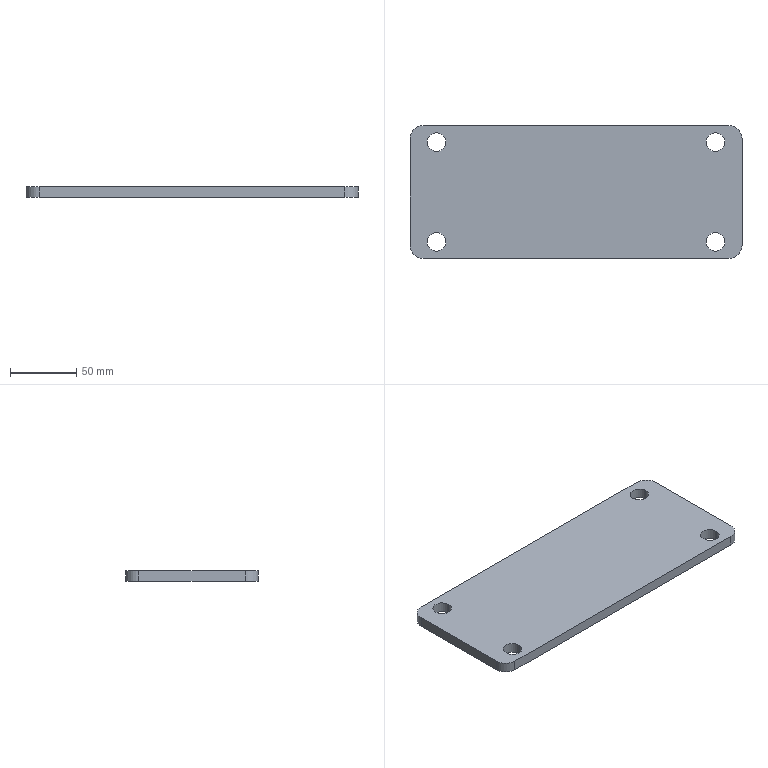Part | SolidWorks | features Chamfer 1, Extrusion 1, Fillet 1, HoleWzd 1 | 1 solid | 18 faces | box 250 x 100 x 8 mm | volume 194387 mm3 | cylinder 12 | plane 6 | commonest cylinder face diameters 14 x8 20 x4
STEP:
#1=CARTESIAN_POINT('',(-112.,37.5,-4.));
#2=VERTEX_POINT('',#1);
#3=CARTESIAN_POINT('',(-98.,37.5,-4.));
#4=VERTEX_POINT('',#3);
#5=CARTESIAN_POINT('',(-105.,37.5,-4.));
#6=DIRECTION('',(0.,0.,1.));
#7=DIRECTION('',(1.,0.,0.));
#8=AXIS2_PLACEMENT_3D('',#5,#6,#7);
#9=CIRCLE('',#8,7.);
#10=EDGE_CURVE('',#2,#4,#9,.T.);
#11=ORIENTED_EDGE('',*,*,#10,.F.);
#12=CARTESIAN_POINT('',(-112.,37.5,4.));
#13=VERTEX_POINT('',#12);
#14=CARTESIAN_POINT('',(-112.,37.5,4.));
#15=DIRECTION('',(0.,0.,1.));
#16=VECTOR('',#15,1000.);
#17=LINE('',#14,#16);
#18=EDGE_CURVE('',#2,#13,#17,.T.);
#19=ORIENTED_EDGE('',*,*,#18,.T.);
#20=CARTESIAN_POINT('',(-98.,37.5,4.));
#21=VERTEX_POINT('',#20);
#22=CARTESIAN_POINT('',(-105.,37.5,4.));
#23=DIRECTION('',(0.,0.,1.));
#24=DIRECTION('',(1.,0.,0.));
#25=AXIS2_PLACEMENT_3D('',#22,#23,#24);
#26=CIRCLE('',#25,7.);
#27=EDGE_CURVE('',#13,#21,#26,.T.);
#28=ORIENTED_EDGE('',*,*,#27,.T.);
#29=CARTESIAN_POINT('',(-98.,37.5,4.));
#30=DIRECTION('',(0.,0.,1.));
#31=VECTOR('',#30,1000.);
#32=LINE('',#29,#31);
#33=EDGE_CURVE('',#4,#21,#32,.T.);
#34=ORIENTED_EDGE('',*,*,#33,.F.);
#35=EDGE_LOOP('',(#11,#19,#28,#34));
#36=FACE_OUTER_BOUND('',#35,.T.);
#37=CARTESIAN_POINT('',(-105.,37.5,4.));
#38=DIRECTION('',(0.,0.,1.));
#39=DIRECTION('',(1.,0.,0.));
#40=AXIS2_PLACEMENT_3D('',#37,#38,#39);
#41=CYLINDRICAL_SURFACE('',#40,7.);
#42=ADVANCED_FACE('',(#36),#41,.F.);
#43=CARTESIAN_POINT('',(98.,37.5,-4.));
#44=VERTEX_POINT('',#43);
#45=CARTESIAN_POINT('',(112.,37.5,-4.));
#46=VERTEX_POINT('',#45);
#47=CARTESIAN_POINT('',(105.,37.5,-4.));
#48=DIRECTION('',(0.,0.,1.));
#49=DIRECTION('',(1.,0.,0.));
#50=AXIS2_PLACEMENT_3D('',#47,#48,#49);
#51=CIRCLE('',#50,7.);
#52=EDGE_CURVE('',#44,#46,#51,.T.);
#53=ORIENTED_EDGE('',*,*,#52,.F.);
#54=CARTESIAN_POINT('',(98.,37.5,4.));
#55=VERTEX_POINT('',#54);
#56=CARTESIAN_POINT('',(98.,37.5,4.));
#57=DIRECTION('',(0.,0.,1.));
#58=VECTOR('',#57,1000.);
#59=LINE('',#56,#58);
#60=EDGE_CURVE('',#44,#55,#59,.T.);
#61=ORIENTED_EDGE('',*,*,#60,.T.);
#62=CARTESIAN_POINT('',(112.,37.5,4.));
#63=VERTEX_POINT('',#62);
#64=CARTESIAN_POINT('',(105.,37.5,4.));
#65=DIRECTION('',(0.,0.,1.));
#66=DIRECTION('',(1.,0.,0.));
#67=AXIS2_PLACEMENT_3D('',#64,#65,#66);
#68=CIRCLE('',#67,7.);
#69=EDGE_CURVE('',#55,#63,#68,.T.);
#70=ORIENTED_EDGE('',*,*,#69,.T.);
#71=CARTESIAN_POINT('',(112.,37.5,4.));
#72=DIRECTION('',(0.,0.,1.));
#73=VECTOR('',#72,1000.);
#74=LINE('',#71,#73);
#75=EDGE_CURVE('',#46,#63,#74,.T.);
#76=ORIENTED_EDGE('',*,*,#75,.F.);
#77=EDGE_LOOP('',(#53,#61,#70,#76));
#78=FACE_OUTER_BOUND('',#77,.T.);
#79=CARTESIAN_POINT('',(105.,37.5,4.));
#80=DIRECTION('',(0.,0.,1.));
#81=DIRECTION('',(1.,0.,0.));
#82=AXIS2_PLACEMENT_3D('',#79,#80,#81);
#83=CYLINDRICAL_SURFACE('',#82,7.);
#84=ADVANCED_FACE('',(#78),#83,.F.);
#85=CARTESIAN_POINT('',(98.,-37.5,-4.));
#86=VERTEX_POINT('',#85);
#87=CARTESIAN_POINT('',(112.,-37.5,-4.));
#88=VERTEX_POINT('',#87);
#89=CARTESIAN_POINT('',(105.,-37.5,-4.));
#90=DIRECTION('',(0.,0.,1.));
#91=DIRECTION('',(1.,0.,0.));
#92=AXIS2_PLACEMENT_3D('',#89,#90,#91);
#93=CIRCLE('',#92,7.);
#94=EDGE_CURVE('',#86,#88,#93,.T.);
#95=ORIENTED_EDGE('',*,*,#94,.F.);
#96=CARTESIAN_POINT('',(98.,-37.5,4.));
#97=VERTEX_POINT('',#96);
#98=CARTESIAN_POINT('',(98.,-37.5,4.));
#99=DIRECTION('',(0.,0.,1.));
#100=VECTOR('',#99,1000.);
#101=LINE('',#98,#100);
#102=EDGE_CURVE('',#86,#97,#101,.T.);
#103=ORIENTED_EDGE('',*,*,#102,.T.);
#104=CARTESIAN_POINT('',(112.,-37.5,4.));
#105=VERTEX_POINT('',#104);
#106=CARTESIAN_POINT('',(105.,-37.5,4.));
#107=DIRECTION('',(0.,0.,1.));
#108=DIRECTION('',(1.,0.,0.));
#109=AXIS2_PLACEMENT_3D('',#106,#107,#108);
#110=CIRCLE('',#109,7.);
#111=EDGE_CURVE('',#97,#105,#110,.T.);
#112=ORIENTED_EDGE('',*,*,#111,.T.);
#113=CARTESIAN_POINT('',(112.,-37.5,4.));
#114=DIRECTION('',(0.,0.,1.));
#115=VECTOR('',#114,1000.);
#116=LINE('',#113,#115);
#117=EDGE_CURVE('',#88,#105,#116,.T.);
#118=ORIENTED_EDGE('',*,*,#117,.F.);
#119=EDGE_LOOP('',(#95,#103,#112,#118));
#120=FACE_OUTER_BOUND('',#119,.T.);
#121=CARTESIAN_POINT('',(105.,-37.5,4.));
#122=DIRECTION('',(0.,0.,1.));
#123=DIRECTION('',(1.,0.,0.));
#124=AXIS2_PLACEMENT_3D('',#121,#122,#123);
#125=CYLINDRICAL_SURFACE('',#124,7.);
#126=ADVANCED_FACE('',(#120),#125,.F.);
#127=CARTESIAN_POINT('',(-112.,-37.5,-4.));
#128=VERTEX_POINT('',#127);
#129=CARTESIAN_POINT('',(-98.,-37.5,-4.));
#130=VERTEX_POINT('',#129);
#131=CARTESIAN_POINT('',(-105.,-37.5,-4.));
#132=DIRECTION('',(0.,0.,1.));
#133=DIRECTION('',(1.,0.,0.));
#134=AXIS2_PLACEMENT_3D('',#131,#132,#133);
#135=CIRCLE('',#134,7.);
#136=EDGE_CURVE('',#128,#130,#135,.T.);
#137=ORIENTED_EDGE('',*,*,#136,.F.);
#138=CARTESIAN_POINT('',(-112.,-37.5,4.));
#139=VERTEX_POINT('',#138);
#140=CARTESIAN_POINT('',(-112.,-37.5,4.));
#141=DIRECTION('',(0.,0.,1.));
#142=VECTOR('',#141,1000.);
#143=LINE('',#140,#142);
#144=EDGE_CURVE('',#128,#139,#143,.T.);
#145=ORIENTED_EDGE('',*,*,#144,.T.);
#146=CARTESIAN_POINT('',(-98.,-37.5,4.));
#147=VERTEX_POINT('',#146);
#148=CARTESIAN_POINT('',(-105.,-37.5,4.));
#149=DIRECTION('',(0.,0.,1.));
#150=DIRECTION('',(1.,0.,0.));
#151=AXIS2_PLACEMENT_3D('',#148,#149,#150);
#152=CIRCLE('',#151,7.);
#153=EDGE_CURVE('',#139,#147,#152,.T.);
#154=ORIENTED_EDGE('',*,*,#153,.T.);
#155=CARTESIAN_POINT('',(-98.,-37.5,4.));
#156=DIRECTION('',(0.,0.,1.));
#157=VECTOR('',#156,1000.);
#158=LINE('',#155,#157);
#159=EDGE_CURVE('',#130,#147,#158,.T.);
#160=ORIENTED_EDGE('',*,*,#159,.F.);
#161=EDGE_LOOP('',(#137,#145,#154,#160));
#162=FACE_OUTER_BOUND('',#161,.T.);
#163=CARTESIAN_POINT('',(-105.,-37.5,4.));
#164=DIRECTION('',(0.,0.,1.));
#165=DIRECTION('',(1.,0.,0.));
#166=AXIS2_PLACEMENT_3D('',#163,#164,#165);
#167=CYLINDRICAL_SURFACE('',#166,7.);
#168=ADVANCED_FACE('',(#162),#167,.F.);
#169=CARTESIAN_POINT('',(-125.,40.,-4.));
#170=VERTEX_POINT('',#169);
#171=CARTESIAN_POINT('',(-125.,-40.,-4.));
#172=VERTEX_POINT('',#171);
#173=CARTESIAN_POINT('',(-125.,-50.,-4.));
#174=DIRECTION('',(0.,-1.,0.));
#175=VECTOR('',#174,1000.);
#176=LINE('',#173,#175);
#177=EDGE_CURVE('',#170,#172,#176,.T.);
#178=ORIENTED_EDGE('',*,*,#177,.T.);
#179=CARTESIAN_POINT('',(-125.,-40.,4.));
#180=VERTEX_POINT('',#179);
#181=CARTESIAN_POINT('',(-125.,-40.,4.));
#182=DIRECTION('',(0.,0.,1.));
#183=VECTOR('',#182,1000.);
#184=LINE('',#181,#183);
#185=EDGE_CURVE('',#172,#180,#184,.T.);
#186=ORIENTED_EDGE('',*,*,#185,.T.);
#187=CARTESIAN_POINT('',(-125.,40.,4.));
#188=VERTEX_POINT('',#187);
#189=CARTESIAN_POINT('',(-125.,-50.,4.));
#190=DIRECTION('',(0.,-1.,0.));
#191=VECTOR('',#190,1000.);
#192=LINE('',#189,#191);
#193=EDGE_CURVE('',#188,#180,#192,.T.);
#194=ORIENTED_EDGE('',*,*,#193,.F.);
#195=CARTESIAN_POINT('',(-125.,40.,4.));
#196=DIRECTION('',(0.,0.,-1.));
#197=VECTOR('',#196,1000.);
#198=LINE('',#195,#197);
#199=EDGE_CURVE('',#188,#170,#198,.T.);
#200=ORIENTED_EDGE('',*,*,#199,.T.);
#201=EDGE_LOOP('',(#178,#186,#194,#200));
#202=FACE_OUTER_BOUND('',#201,.T.);
#203=CARTESIAN_POINT('',(-125.,-50.,4.));
#204=DIRECTION('',(1.,0.,0.));
#205=DIRECTION('',(0.,0.,-1.));
#206=AXIS2_PLACEMENT_3D('',#203,#204,#205);
#207=PLANE('',#206);
#208=ADVANCED_FACE('',(#202),#207,.F.);
#209=CARTESIAN_POINT('',(-115.,-50.,-4.));
#210=VERTEX_POINT('',#209);
#211=CARTESIAN_POINT('',(115.,-50.,-4.));
#212=VERTEX_POINT('',#211);
#213=CARTESIAN_POINT('',(125.,-50.,-4.));
#214=DIRECTION('',(1.,0.,0.));
#215=VECTOR('',#214,1000.);
#216=LINE('',#213,#215);
#217=EDGE_CURVE('',#210,#212,#216,.T.);
#218=ORIENTED_EDGE('',*,*,#217,.T.);
#219=CARTESIAN_POINT('',(115.,-50.,4.));
#220=VERTEX_POINT('',#219);
#221=CARTESIAN_POINT('',(115.,-50.,4.));
#222=DIRECTION('',(0.,0.,1.));
#223=VECTOR('',#222,1000.);
#224=LINE('',#221,#223);
#225=EDGE_CURVE('',#212,#220,#224,.T.);
#226=ORIENTED_EDGE('',*,*,#225,.T.);
#227=CARTESIAN_POINT('',(-115.,-50.,4.));
#228=VERTEX_POINT('',#227);
#229=CARTESIAN_POINT('',(125.,-50.,4.));
#230=DIRECTION('',(1.,0.,0.));
#231=VECTOR('',#230,1000.);
#232=LINE('',#229,#231);
#233=EDGE_CURVE('',#228,#220,#232,.T.);
#234=ORIENTED_EDGE('',*,*,#233,.F.);
#235=CARTESIAN_POINT('',(-115.,-50.,4.));
#236=DIRECTION('',(0.,0.,-1.));
#237=VECTOR('',#236,1000.);
#238=LINE('',#235,#237);
#239=EDGE_CURVE('',#228,#210,#238,.T.);
#240=ORIENTED_EDGE('',*,*,#239,.T.);
#241=EDGE_LOOP('',(#218,#226,#234,#240));
#242=FACE_OUTER_BOUND('',#241,.T.);
#243=CARTESIAN_POINT('',(125.,-50.,4.));
#244=DIRECTION('',(0.,1.,0.));
#245=DIRECTION('',(-1.,0.,0.));
#246=AXIS2_PLACEMENT_3D('',#243,#244,#245);
#247=PLANE('',#246);
#248=ADVANCED_FACE('',(#242),#247,.F.);
#249=CARTESIAN_POINT('',(125.,-40.,-4.));
#250=VERTEX_POINT('',#249);
#251=CARTESIAN_POINT('',(125.,40.,-4.));
#252=VERTEX_POINT('',#251);
#253=CARTESIAN_POINT('',(125.,-50.,-4.));
#254=DIRECTION('',(0.,1.,0.));
#255=VECTOR('',#254,1000.);
#256=LINE('',#253,#255);
#257=EDGE_CURVE('',#250,#252,#256,.T.);
#258=ORIENTED_EDGE('',*,*,#257,.T.);
#259=CARTESIAN_POINT('',(125.,40.,4.));
#260=VERTEX_POINT('',#259);
#261=CARTESIAN_POINT('',(125.,40.,4.));
#262=DIRECTION('',(0.,0.,1.));
#263=VECTOR('',#262,1000.);
#264=LINE('',#261,#263);
#265=EDGE_CURVE('',#252,#260,#264,.T.);
#266=ORIENTED_EDGE('',*,*,#265,.T.);
#267=CARTESIAN_POINT('',(125.,-40.,4.));
#268=VERTEX_POINT('',#267);
#269=CARTESIAN_POINT('',(125.,-50.,4.));
#270=DIRECTION('',(0.,1.,0.));
#271=VECTOR('',#270,1000.);
#272=LINE('',#269,#271);
#273=EDGE_CURVE('',#268,#260,#272,.T.);
#274=ORIENTED_EDGE('',*,*,#273,.F.);
#275=CARTESIAN_POINT('',(125.,-40.,4.));
#276=DIRECTION('',(0.,0.,-1.));
#277=VECTOR('',#276,1000.);
#278=LINE('',#275,#277);
#279=EDGE_CURVE('',#268,#250,#278,.T.);
#280=ORIENTED_EDGE('',*,*,#279,.T.);
#281=EDGE_LOOP('',(#258,#266,#274,#280));
#282=FACE_OUTER_BOUND('',#281,.T.);
#283=CARTESIAN_POINT('',(125.,-50.,4.));
#284=DIRECTION('',(-1.,0.,0.));
#285=DIRECTION('',(0.,0.,1.));
#286=AXIS2_PLACEMENT_3D('',#283,#284,#285);
#287=PLANE('',#286);
#288=ADVANCED_FACE('',(#282),#287,.F.);
#289=CARTESIAN_POINT('',(115.,50.,4.));
#290=VERTEX_POINT('',#289);
#291=CARTESIAN_POINT('',(-115.,50.,4.));
#292=VERTEX_POINT('',#291);
#293=CARTESIAN_POINT('',(125.,50.,4.));
#294=DIRECTION('',(-1.,0.,0.));
#295=VECTOR('',#294,1000.);
#296=LINE('',#293,#295);
#297=EDGE_CURVE('',#290,#292,#296,.T.);
#298=ORIENTED_EDGE('',*,*,#297,.F.);
#299=CARTESIAN_POINT('',(115.,50.,-4.));
#300=VERTEX_POINT('',#299);
#301=CARTESIAN_POINT('',(115.,50.,4.));
#302=DIRECTION('',(0.,0.,-1.));
#303=VECTOR('',#302,1000.);
#304=LINE('',#301,#303);
#305=EDGE_CURVE('',#290,#300,#304,.T.);
#306=ORIENTED_EDGE('',*,*,#305,.T.);
#307=CARTESIAN_POINT('',(-115.,50.,-4.));
#308=VERTEX_POINT('',#307);
#309=CARTESIAN_POINT('',(125.,50.,-4.));
#310=DIRECTION('',(-1.,0.,0.));
#311=VECTOR('',#310,1000.);
#312=LINE('',#309,#311);
#313=EDGE_CURVE('',#300,#308,#312,.T.);
#314=ORIENTED_EDGE('',*,*,#313,.T.);
#315=CARTESIAN_POINT('',(-115.,50.,4.));
#316=DIRECTION('',(0.,0.,1.));
#317=VECTOR('',#316,1000.);
#318=LINE('',#315,#317);
#319=EDGE_CURVE('',#308,#292,#318,.T.);
#320=ORIENTED_EDGE('',*,*,#319,.T.);
#321=EDGE_LOOP('',(#298,#306,#314,#320));
#322=FACE_OUTER_BOUND('',#321,.T.);
#323=CARTESIAN_POINT('',(125.,50.,4.));
#324=DIRECTION('',(0.,-1.,0.));
#325=DIRECTION('',(1.,0.,0.));
#326=AXIS2_PLACEMENT_3D('',#323,#324,#325);
#327=PLANE('',#326);
#328=ADVANCED_FACE('',(#322),#327,.F.);
#329=CARTESIAN_POINT('',(-105.,37.5,4.));
#330=DIRECTION('',(0.,0.,1.));
#331=DIRECTION('',(1.,0.,0.));
#332=AXIS2_PLACEMENT_3D('',#329,#330,#331);
#333=CIRCLE('',#332,7.);
#334=EDGE_CURVE('',#21,#13,#333,.T.);
#335=ORIENTED_EDGE('',*,*,#334,.F.);
#336=ORIENTED_EDGE('',*,*,#27,.F.);
#337=EDGE_LOOP('',(#335,#336));
#338=FACE_BOUND('',#337,.T.);
#339=CARTESIAN_POINT('',(105.,37.5,4.));
#340=DIRECTION('',(0.,0.,1.));
#341=DIRECTION('',(1.,0.,0.));
#342=AXIS2_PLACEMENT_3D('',#339,#340,#341);
#343=CIRCLE('',#342,7.);
#344=EDGE_CURVE('',#63,#55,#343,.T.);
#345=ORIENTED_EDGE('',*,*,#344,.F.);
#346=ORIENTED_EDGE('',*,*,#69,.F.);
#347=EDGE_LOOP('',(#345,#346));
#348=FACE_BOUND('',#347,.T.);
#349=CARTESIAN_POINT('',(105.,-37.5,4.));
#350=DIRECTION('',(0.,0.,1.));
#351=DIRECTION('',(1.,0.,0.));
#352=AXIS2_PLACEMENT_3D('',#349,#350,#351);
#353=CIRCLE('',#352,7.);
#354=EDGE_CURVE('',#105,#97,#353,.T.);
#355=ORIENTED_EDGE('',*,*,#354,.F.);
#356=ORIENTED_EDGE('',*,*,#111,.F.);
#357=EDGE_LOOP('',(#355,#356));
#358=FACE_BOUND('',#357,.T.);
#359=CARTESIAN_POINT('',(-105.,-37.5,4.));
#360=DIRECTION('',(0.,0.,1.));
#361=DIRECTION('',(1.,0.,0.));
#362=AXIS2_PLACEMENT_3D('',#359,#360,#361);
#363=CIRCLE('',#362,7.);
#364=EDGE_CURVE('',#147,#139,#363,.T.);
#365=ORIENTED_EDGE('',*,*,#364,.F.);
#366=ORIENTED_EDGE('',*,*,#153,.F.);
#367=EDGE_LOOP('',(#365,#366));
#368=FACE_BOUND('',#367,.T.);
#369=ORIENTED_EDGE('',*,*,#273,.T.);
#370=CARTESIAN_POINT('',(115.,40.,4.));
#371=DIRECTION('',(0.,0.,1.));
#372=DIRECTION('',(1.,0.,0.));
#373=AXIS2_PLACEMENT_3D('',#370,#371,#372);
#374=CIRCLE('',#373,10.);
#375=EDGE_CURVE('',#260,#290,#374,.T.);
#376=ORIENTED_EDGE('',*,*,#375,.T.);
#377=ORIENTED_EDGE('',*,*,#297,.T.);
#378=CARTESIAN_POINT('',(-115.,40.,4.));
#379=DIRECTION('',(0.,0.,1.));
#380=DIRECTION('',(1.,0.,0.));
#381=AXIS2_PLACEMENT_3D('',#378,#379,#380);
#382=CIRCLE('',#381,10.);
#383=EDGE_CURVE('',#292,#188,#382,.T.);
#384=ORIENTED_EDGE('',*,*,#383,.T.);
#385=ORIENTED_EDGE('',*,*,#193,.T.);
#386=CARTESIAN_POINT('',(-115.,-40.,4.));
#387=DIRECTION('',(0.,0.,1.));
#388=DIRECTION('',(1.,0.,0.));
#389=AXIS2_PLACEMENT_3D('',#386,#387,#388);
#390=CIRCLE('',#389,10.);
#391=EDGE_CURVE('',#180,#228,#390,.T.);
#392=ORIENTED_EDGE('',*,*,#391,.T.);
#393=ORIENTED_EDGE('',*,*,#233,.T.);
#394=CARTESIAN_POINT('',(115.,-40.,4.));
#395=DIRECTION('',(0.,0.,1.));
#396=DIRECTION('',(1.,0.,0.));
#397=AXIS2_PLACEMENT_3D('',#394,#395,#396);
#398=CIRCLE('',#397,10.);
#399=EDGE_CURVE('',#220,#268,#398,.T.);
#400=ORIENTED_EDGE('',*,*,#399,.T.);
#401=EDGE_LOOP('',(#369,#376,#377,#384,#385,#392,#393,#400));
#402=FACE_OUTER_BOUND('',#401,.T.);
#403=CARTESIAN_POINT('',(0.,0.,4.));
#404=DIRECTION('',(0.,0.,1.));
#405=DIRECTION('',(1.,0.,0.));
#406=AXIS2_PLACEMENT_3D('',#403,#404,#405);
#407=PLANE('',#406);
#408=ADVANCED_FACE('',(#338,#348,#358,#368,#402),#407,.T.);
#409=CARTESIAN_POINT('',(-105.,37.5,-4.));
#410=DIRECTION('',(0.,0.,1.));
#411=DIRECTION('',(1.,0.,0.));
#412=AXIS2_PLACEMENT_3D('',#409,#410,#411);
#413=CIRCLE('',#412,7.);
#414=EDGE_CURVE('',#4,#2,#413,.T.);
#415=ORIENTED_EDGE('',*,*,#414,.T.);
#416=ORIENTED_EDGE('',*,*,#10,.T.);
#417=EDGE_LOOP('',(#415,#416));
#418=FACE_BOUND('',#417,.T.);
#419=CARTESIAN_POINT('',(105.,37.5,-4.));
#420=DIRECTION('',(0.,0.,1.));
#421=DIRECTION('',(1.,0.,0.));
#422=AXIS2_PLACEMENT_3D('',#419,#420,#421);
#423=CIRCLE('',#422,7.);
#424=EDGE_CURVE('',#46,#44,#423,.T.);
#425=ORIENTED_EDGE('',*,*,#424,.T.);
#426=ORIENTED_EDGE('',*,*,#52,.T.);
#427=EDGE_LOOP('',(#425,#426));
#428=FACE_BOUND('',#427,.T.);
#429=CARTESIAN_POINT('',(105.,-37.5,-4.));
#430=DIRECTION('',(0.,0.,1.));
#431=DIRECTION('',(1.,0.,0.));
#432=AXIS2_PLACEMENT_3D('',#429,#430,#431);
#433=CIRCLE('',#432,7.);
#434=EDGE_CURVE('',#88,#86,#433,.T.);
#435=ORIENTED_EDGE('',*,*,#434,.T.);
#436=ORIENTED_EDGE('',*,*,#94,.T.);
#437=EDGE_LOOP('',(#435,#436));
#438=FACE_BOUND('',#437,.T.);
#439=CARTESIAN_POINT('',(-105.,-37.5,-4.));
#440=DIRECTION('',(0.,0.,1.));
#441=DIRECTION('',(1.,0.,0.));
#442=AXIS2_PLACEMENT_3D('',#439,#440,#441);
#443=CIRCLE('',#442,7.);
#444=EDGE_CURVE('',#130,#128,#443,.T.);
#445=ORIENTED_EDGE('',*,*,#444,.T.);
#446=ORIENTED_EDGE('',*,*,#136,.T.);
#447=EDGE_LOOP('',(#445,#446));
#448=FACE_BOUND('',#447,.T.);
#449=ORIENTED_EDGE('',*,*,#313,.F.);
#450=CARTESIAN_POINT('',(115.,40.,-4.));
#451=DIRECTION('',(0.,0.,-1.));
#452=DIRECTION('',(1.,0.,0.));
#453=AXIS2_PLACEMENT_3D('',#450,#451,#452);
#454=CIRCLE('',#453,10.);
#455=EDGE_CURVE('',#300,#252,#454,.T.);
#456=ORIENTED_EDGE('',*,*,#455,.T.);
#457=ORIENTED_EDGE('',*,*,#257,.F.);
#458=CARTESIAN_POINT('',(115.,-40.,-4.));
#459=DIRECTION('',(0.,0.,-1.));
#460=DIRECTION('',(1.,0.,0.));
#461=AXIS2_PLACEMENT_3D('',#458,#459,#460);
#462=CIRCLE('',#461,10.);
#463=EDGE_CURVE('',#250,#212,#462,.T.);
#464=ORIENTED_EDGE('',*,*,#463,.T.);
#465=ORIENTED_EDGE('',*,*,#217,.F.);
#466=CARTESIAN_POINT('',(-115.,-40.,-4.));
#467=DIRECTION('',(0.,0.,-1.));
#468=DIRECTION('',(1.,0.,0.));
#469=AXIS2_PLACEMENT_3D('',#466,#467,#468);
#470=CIRCLE('',#469,10.);
#471=EDGE_CURVE('',#210,#172,#470,.T.);
#472=ORIENTED_EDGE('',*,*,#471,.T.);
#473=ORIENTED_EDGE('',*,*,#177,.F.);
#474=CARTESIAN_POINT('',(-115.,40.,-4.));
#475=DIRECTION('',(0.,0.,-1.));
#476=DIRECTION('',(1.,0.,0.));
#477=AXIS2_PLACEMENT_3D('',#474,#475,#476);
#478=CIRCLE('',#477,10.);
#479=EDGE_CURVE('',#170,#308,#478,.T.);
#480=ORIENTED_EDGE('',*,*,#479,.T.);
#481=EDGE_LOOP('',(#449,#456,#457,#464,#465,#472,#473,#480));
#482=FACE_OUTER_BOUND('',#481,.T.);
#483=CARTESIAN_POINT('',(0.,0.,-4.));
#484=DIRECTION('',(0.,0.,1.));
#485=DIRECTION('',(1.,0.,0.));
#486=AXIS2_PLACEMENT_3D('',#483,#484,#485);
#487=PLANE('',#486);
#488=ADVANCED_FACE('',(#418,#428,#438,#448,#482),#487,.F.);
#489=ORIENTED_EDGE('',*,*,#144,.F.);
#490=ORIENTED_EDGE('',*,*,#444,.F.);
#491=ORIENTED_EDGE('',*,*,#159,.T.);
#492=ORIENTED_EDGE('',*,*,#364,.T.);
#493=EDGE_LOOP('',(#489,#490,#491,#492));
#494=FACE_OUTER_BOUND('',#493,.T.);
#495=CARTESIAN_POINT('',(-105.,-37.5,4.));
#496=DIRECTION('',(0.,0.,1.));
#497=DIRECTION('',(1.,0.,0.));
#498=AXIS2_PLACEMENT_3D('',#495,#496,#497);
#499=CYLINDRICAL_SURFACE('',#498,7.);
#500=ADVANCED_FACE('',(#494),#499,.F.);
#501=ORIENTED_EDGE('',*,*,#102,.F.);
#502=ORIENTED_EDGE('',*,*,#434,.F.);
#503=ORIENTED_EDGE('',*,*,#117,.T.);
#504=ORIENTED_EDGE('',*,*,#354,.T.);
#505=EDGE_LOOP('',(#501,#502,#503,#504));
#506=FACE_OUTER_BOUND('',#505,.T.);
#507=CARTESIAN_POINT('',(105.,-37.5,4.));
#508=DIRECTION('',(0.,0.,1.));
#509=DIRECTION('',(1.,0.,0.));
#510=AXIS2_PLACEMENT_3D('',#507,#508,#509);
#511=CYLINDRICAL_SURFACE('',#510,7.);
#512=ADVANCED_FACE('',(#506),#511,.F.);
#513=ORIENTED_EDGE('',*,*,#60,.F.);
#514=ORIENTED_EDGE('',*,*,#424,.F.);
#515=ORIENTED_EDGE('',*,*,#75,.T.);
#516=ORIENTED_EDGE('',*,*,#344,.T.);
#517=EDGE_LOOP('',(#513,#514,#515,#516));
#518=FACE_OUTER_BOUND('',#517,.T.);
#519=CARTESIAN_POINT('',(105.,37.5,4.));
#520=DIRECTION('',(0.,0.,1.));
#521=DIRECTION('',(1.,0.,0.));
#522=AXIS2_PLACEMENT_3D('',#519,#520,#521);
#523=CYLINDRICAL_SURFACE('',#522,7.);
#524=ADVANCED_FACE('',(#518),#523,.F.);
#525=ORIENTED_EDGE('',*,*,#18,.F.);
#526=ORIENTED_EDGE('',*,*,#414,.F.);
#527=ORIENTED_EDGE('',*,*,#33,.T.);
#528=ORIENTED_EDGE('',*,*,#334,.T.);
#529=EDGE_LOOP('',(#525,#526,#527,#528));
#530=FACE_OUTER_BOUND('',#529,.T.);
#531=CARTESIAN_POINT('',(-105.,37.5,4.));
#532=DIRECTION('',(0.,0.,1.));
#533=DIRECTION('',(1.,0.,0.));
#534=AXIS2_PLACEMENT_3D('',#531,#532,#533);
#535=CYLINDRICAL_SURFACE('',#534,7.);
#536=ADVANCED_FACE('',(#530),#535,.F.);
#537=ORIENTED_EDGE('',*,*,#375,.F.);
#538=ORIENTED_EDGE('',*,*,#265,.F.);
#539=ORIENTED_EDGE('',*,*,#455,.F.);
#540=ORIENTED_EDGE('',*,*,#305,.F.);
#541=EDGE_LOOP('',(#537,#538,#539,#540));
#542=FACE_OUTER_BOUND('',#541,.T.);
#543=CARTESIAN_POINT('',(115.,40.,4.));
#544=DIRECTION('',(0.,0.,-1.));
#545=DIRECTION('',(-1.,0.,0.));
#546=AXIS2_PLACEMENT_3D('',#543,#544,#545);
#547=CYLINDRICAL_SURFACE('',#546,10.);
#548=ADVANCED_FACE('',(#542),#547,.T.);
#549=ORIENTED_EDGE('',*,*,#399,.F.);
#550=ORIENTED_EDGE('',*,*,#225,.F.);
#551=ORIENTED_EDGE('',*,*,#463,.F.);
#552=ORIENTED_EDGE('',*,*,#279,.F.);
#553=EDGE_LOOP('',(#549,#550,#551,#552));
#554=FACE_OUTER_BOUND('',#553,.T.);
#555=CARTESIAN_POINT('',(115.,-40.,4.));
#556=DIRECTION('',(0.,0.,-1.));
#557=DIRECTION('',(-1.,0.,0.));
#558=AXIS2_PLACEMENT_3D('',#555,#556,#557);
#559=CYLINDRICAL_SURFACE('',#558,10.);
#560=ADVANCED_FACE('',(#554),#559,.T.);
#561=ORIENTED_EDGE('',*,*,#391,.F.);
#562=ORIENTED_EDGE('',*,*,#185,.F.);
#563=ORIENTED_EDGE('',*,*,#471,.F.);
#564=ORIENTED_EDGE('',*,*,#239,.F.);
#565=EDGE_LOOP('',(#561,#562,#563,#564));
#566=FACE_OUTER_BOUND('',#565,.T.);
#567=CARTESIAN_POINT('',(-115.,-40.,4.));
#568=DIRECTION('',(0.,0.,-1.));
#569=DIRECTION('',(-1.,0.,0.));
#570=AXIS2_PLACEMENT_3D('',#567,#568,#569);
#571=CYLINDRICAL_SURFACE('',#570,10.);
#572=ADVANCED_FACE('',(#566),#571,.T.);
#573=ORIENTED_EDGE('',*,*,#383,.F.);
#574=ORIENTED_EDGE('',*,*,#319,.F.);
#575=ORIENTED_EDGE('',*,*,#479,.F.);
#576=ORIENTED_EDGE('',*,*,#199,.F.);
#577=EDGE_LOOP('',(#573,#574,#575,#576));
#578=FACE_OUTER_BOUND('',#577,.T.);
#579=CARTESIAN_POINT('',(-115.,40.,4.));
#580=DIRECTION('',(0.,0.,-1.));
#581=DIRECTION('',(-1.,0.,0.));
#582=AXIS2_PLACEMENT_3D('',#579,#580,#581);
#583=CYLINDRICAL_SURFACE('',#582,10.);
#584=ADVANCED_FACE('',(#578),#583,.T.);
#585=CLOSED_SHELL('',(#42,#84,#126,#168,#208,#248,#288,#328,#408,#488,#500,#512,#524,#536,#548,#560,#572,#584));
#586=MANIFOLD_SOLID_BREP('',#585);
#587=CARTESIAN_POINT('',(0.,0.,0.));
#588=DIRECTION('',(0.,0.,1.));
#589=DIRECTION('',(1.,0.,0.));
#590=AXIS2_PLACEMENT_3D('',#587,#588,#589);
#591=(LENGTH_UNIT()NAMED_UNIT(*)SI_UNIT(.MILLI.,.METRE.));
#592=UNCERTAINTY_MEASURE_WITH_UNIT(LENGTH_MEASURE(0.00001),#591,'','');
#593=(NAMED_UNIT(*)PLANE_ANGLE_UNIT()SI_UNIT($,.RADIAN.));
#594=(NAMED_UNIT(*)SI_UNIT($,.STERADIAN.)SOLID_ANGLE_UNIT());
#595=(GEOMETRIC_REPRESENTATION_CONTEXT(3)GLOBAL_UNCERTAINTY_ASSIGNED_CONTEXT((#592))GLOBAL_UNIT_ASSIGNED_CONTEXT((#591,#593,#594))REPRESENTATION_CONTEXT('',''));
#596=ADVANCED_BREP_SHAPE_REPRESENTATION('',(#586,#590),#595);